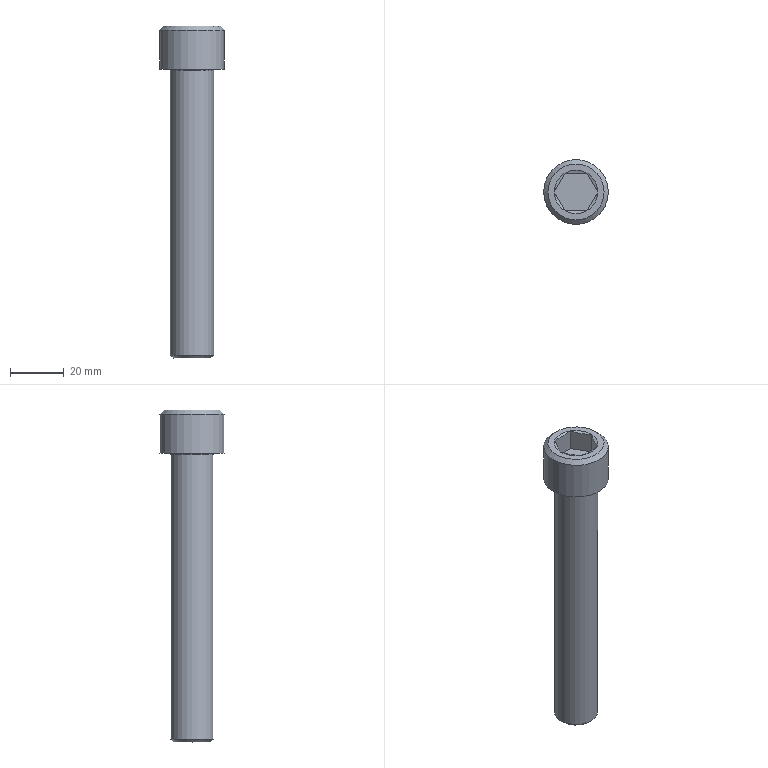Part | STEP file | solid 50 | 1 solid | 21 faces | box 24 x 24 x 123 mm | volume 27276 mm3 | plane 10 | sphere 6 | cylinder 2 | cone 2 | torus 1 | commonest cylinder face diameters 16 x1 24 x1